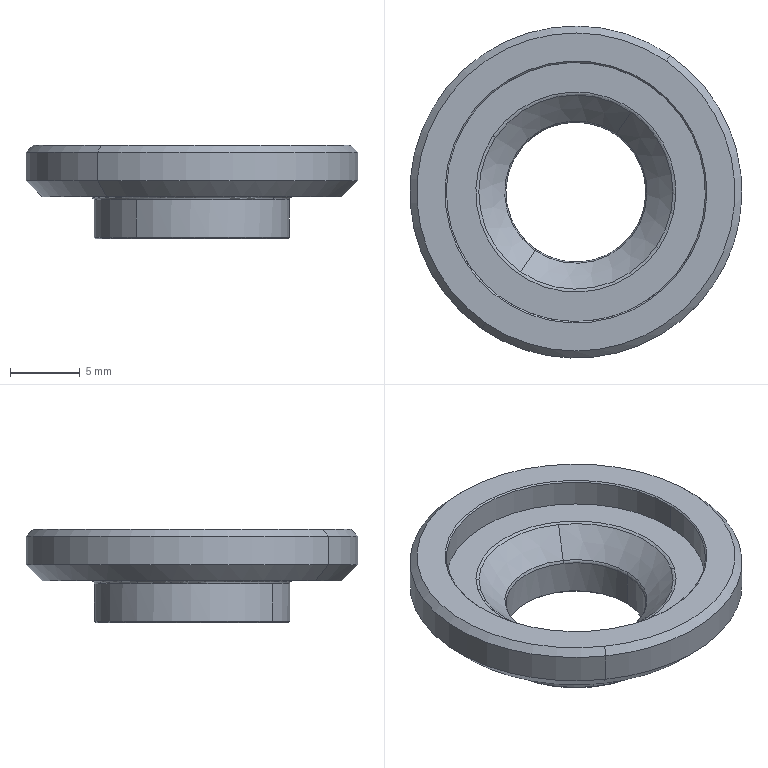Part | SolidWorks | features BaseBody 1 | 1 solid | 36 faces | box 23.8 x 23.8 x 6.7 mm | volume 1063 mm3 | cone 14 | cylinder 10 | torus 8 | plane 4 | commonest cylinder face diameters 14 x3 23.8 x3 10.04 x2 18.57 x2
STEP:
#1=CARTESIAN_POINT('',(85.216,-198.027,4.7));
#2=VERTEX_POINT('',#1);
#3=CARTESIAN_POINT('',(97.083,-206.078,4.7));
#4=VERTEX_POINT('',#3);
#5=CARTESIAN_POINT('',(91.15,-202.053,4.7));
#6=DIRECTION('',(0.,0.,1.));
#7=DIRECTION('',(-0.8275,0.5614,0.));
#8=AXIS2_PLACEMENT_3D('',#5,#6,#7);
#9=CIRCLE('',#8,7.17);
#10=EDGE_CURVE('',#2,#4,#9,.T.);
#11=ORIENTED_EDGE('',*,*,#10,.T.);
#12=CARTESIAN_POINT('',(96.907,-205.959,4.612));
#13=VERTEX_POINT('',#12);
#14=CARTESIAN_POINT('',(97.083,-206.078,4.4));
#15=DIRECTION('',(0.5614,0.8275,0.));
#16=DIRECTION('',(-0.5851,0.397,0.7071));
#17=AXIS2_PLACEMENT_3D('',#14,#15,#16);
#18=CIRCLE('',#17,0.3);
#19=EDGE_CURVE('',#13,#4,#18,.T.);
#20=ORIENTED_EDGE('',*,*,#19,.F.);
#21=CARTESIAN_POINT('',(87.195,-207.777,4.612));
#22=VERTEX_POINT('',#21);
#23=CARTESIAN_POINT('',(91.15,-202.053,4.612));
#24=DIRECTION('',(0.,0.,1.));
#25=DIRECTION('',(-0.5684,-0.8228,0.));
#26=AXIS2_PLACEMENT_3D('',#23,#24,#25);
#27=CIRCLE('',#26,6.958);
#28=EDGE_CURVE('',#22,#13,#27,.T.);
#29=ORIENTED_EDGE('',*,*,#28,.F.);
#30=CARTESIAN_POINT('',(85.392,-198.147,4.612));
#31=VERTEX_POINT('',#30);
#32=CARTESIAN_POINT('',(91.15,-202.053,4.612));
#33=DIRECTION('',(0.,0.,1.));
#34=DIRECTION('',(-0.8275,0.5614,0.));
#35=AXIS2_PLACEMENT_3D('',#32,#33,#34);
#36=CIRCLE('',#35,6.958);
#37=EDGE_CURVE('',#31,#22,#36,.T.);
#38=ORIENTED_EDGE('',*,*,#37,.F.);
#39=CARTESIAN_POINT('',(85.216,-198.027,4.4));
#40=DIRECTION('',(0.5614,0.8275,0.));
#41=DIRECTION('',(0.,0.,1.));
#42=AXIS2_PLACEMENT_3D('',#39,#40,#41);
#43=CIRCLE('',#42,0.3);
#44=EDGE_CURVE('',#2,#31,#43,.T.);
#45=ORIENTED_EDGE('',*,*,#44,.F.);
#46=EDGE_LOOP('',(#11,#20,#29,#38,#45));
#47=FACE_OUTER_BOUND('',#46,.T.);
#48=CARTESIAN_POINT('',(91.15,-202.053,4.4));
#49=DIRECTION('',(0.,0.,-1.));
#50=DIRECTION('',(0.8275,-0.5614,0.));
#51=AXIS2_PLACEMENT_3D('',#48,#49,#50);
#52=TOROIDAL_SURFACE('',#51,7.17,0.3);
#53=ADVANCED_FACE('',(#47),#52,.T.);
#54=ORIENTED_EDGE('',*,*,#44,.T.);
#55=CARTESIAN_POINT('',(95.104,-196.328,4.612));
#56=VERTEX_POINT('',#55);
#57=CARTESIAN_POINT('',(91.15,-202.053,4.612));
#58=DIRECTION('',(0.,0.,1.));
#59=DIRECTION('',(0.5684,0.8228,0.));
#60=AXIS2_PLACEMENT_3D('',#57,#58,#59);
#61=CIRCLE('',#60,6.958);
#62=EDGE_CURVE('',#56,#31,#61,.T.);
#63=ORIENTED_EDGE('',*,*,#62,.F.);
#64=CARTESIAN_POINT('',(91.15,-202.053,4.612));
#65=DIRECTION('',(0.,0.,1.));
#66=DIRECTION('',(0.8275,-0.5614,0.));
#67=AXIS2_PLACEMENT_3D('',#64,#65,#66);
#68=CIRCLE('',#67,6.958);
#69=EDGE_CURVE('',#13,#56,#68,.T.);
#70=ORIENTED_EDGE('',*,*,#69,.F.);
#71=ORIENTED_EDGE('',*,*,#19,.T.);
#72=CARTESIAN_POINT('',(91.15,-202.053,4.7));
#73=DIRECTION('',(0.,0.,1.));
#74=DIRECTION('',(0.8275,-0.5614,0.));
#75=AXIS2_PLACEMENT_3D('',#72,#73,#74);
#76=CIRCLE('',#75,7.17);
#77=EDGE_CURVE('',#4,#2,#76,.T.);
#78=ORIENTED_EDGE('',*,*,#77,.T.);
#79=EDGE_LOOP('',(#54,#63,#70,#71,#78));
#80=FACE_OUTER_BOUND('',#79,.T.);
#81=CARTESIAN_POINT('',(91.15,-202.053,4.4));
#82=DIRECTION('',(0.,0.,-1.));
#83=DIRECTION('',(-0.8275,0.5614,0.));
#84=AXIS2_PLACEMENT_3D('',#81,#82,#83);
#85=TOROIDAL_SURFACE('',#84,7.17,0.3);
#86=ADVANCED_FACE('',(#80),#85,.T.);
#87=ORIENTED_EDGE('',*,*,#77,.F.);
#88=ORIENTED_EDGE('',*,*,#10,.F.);
#89=EDGE_LOOP('',(#87,#88));
#90=FACE_BOUND('',#89,.T.);
#91=CARTESIAN_POINT('',(100.428,-202.4,4.7));
#92=VERTEX_POINT('',#91);
#93=CARTESIAN_POINT('',(81.871,-201.705,4.7));
#94=VERTEX_POINT('',#93);
#95=CARTESIAN_POINT('',(91.15,-202.053,4.7));
#96=DIRECTION('',(0.,0.,-1.));
#97=DIRECTION('',(0.9993,-0.03741,0.));
#98=AXIS2_PLACEMENT_3D('',#95,#96,#97);
#99=CIRCLE('',#98,9.285);
#100=EDGE_CURVE('',#92,#94,#99,.T.);
#101=ORIENTED_EDGE('',*,*,#100,.F.);
#102=CARTESIAN_POINT('',(91.15,-202.053,4.7));
#103=DIRECTION('',(0.,0.,-1.));
#104=DIRECTION('',(-0.9993,0.03741,0.));
#105=AXIS2_PLACEMENT_3D('',#102,#103,#104);
#106=CIRCLE('',#105,9.285);
#107=EDGE_CURVE('',#94,#92,#106,.T.);
#108=ORIENTED_EDGE('',*,*,#107,.F.);
#109=EDGE_LOOP('',(#101,#108));
#110=FACE_OUTER_BOUND('',#109,.T.);
#111=CARTESIAN_POINT('',(110.022,-194.263,4.7));
#112=DIRECTION('',(0.,0.,1.));
#113=DIRECTION('',(1.,0.,0.));
#114=AXIS2_PLACEMENT_3D('',#111,#112,#113);
#115=PLANE('',#114);
#116=ADVANCED_FACE('',(#90,#110),#115,.T.);
#117=CARTESIAN_POINT('',(81.871,-201.705,6.6));
#118=VERTEX_POINT('',#117);
#119=CARTESIAN_POINT('',(81.871,-201.705,6.6));
#120=DIRECTION('',(0.,0.,-1.));
#121=VECTOR('',#120,1000.);
#122=LINE('',#119,#121);
#123=EDGE_CURVE('',#118,#94,#122,.T.);
#124=ORIENTED_EDGE('',*,*,#123,.T.);
#125=ORIENTED_EDGE('',*,*,#107,.T.);
#126=CARTESIAN_POINT('',(100.428,-202.4,6.6));
#127=VERTEX_POINT('',#126);
#128=CARTESIAN_POINT('',(100.428,-202.4,6.6));
#129=DIRECTION('',(0.,0.,-1.));
#130=VECTOR('',#129,1000.);
#131=LINE('',#128,#130);
#132=EDGE_CURVE('',#127,#92,#131,.T.);
#133=ORIENTED_EDGE('',*,*,#132,.F.);
#134=CARTESIAN_POINT('',(91.15,-202.053,6.6));
#135=DIRECTION('',(0.,0.,1.));
#136=DIRECTION('',(0.9993,-0.03741,0.));
#137=AXIS2_PLACEMENT_3D('',#134,#135,#136);
#138=CIRCLE('',#137,9.285);
#139=EDGE_CURVE('',#127,#118,#138,.T.);
#140=ORIENTED_EDGE('',*,*,#139,.T.);
#141=EDGE_LOOP('',(#124,#125,#133,#140));
#142=FACE_OUTER_BOUND('',#141,.T.);
#143=CARTESIAN_POINT('',(91.15,-202.053,6.7));
#144=DIRECTION('',(0.,0.,1.));
#145=DIRECTION('',(0.9993,-0.03741,0.));
#146=AXIS2_PLACEMENT_3D('',#143,#144,#145);
#147=CYLINDRICAL_SURFACE('',#146,9.285);
#148=ADVANCED_FACE('',(#142),#147,.F.);
#149=CARTESIAN_POINT('',(81.771,-201.702,6.7));
#150=VERTEX_POINT('',#149);
#151=CARTESIAN_POINT('',(81.771,-201.702,6.7));
#152=DIRECTION('',(0.7066,-0.02645,-0.7071));
#153=VECTOR('',#152,1000.);
#154=LINE('',#151,#153);
#155=EDGE_CURVE('',#150,#118,#154,.T.);
#156=ORIENTED_EDGE('',*,*,#155,.T.);
#157=ORIENTED_EDGE('',*,*,#139,.F.);
#158=CARTESIAN_POINT('',(100.528,-202.404,6.7));
#159=VERTEX_POINT('',#158);
#160=CARTESIAN_POINT('',(100.528,-202.404,6.7));
#161=DIRECTION('',(-0.7066,0.02645,-0.7071));
#162=VECTOR('',#161,1000.);
#163=LINE('',#160,#162);
#164=EDGE_CURVE('',#159,#127,#163,.T.);
#165=ORIENTED_EDGE('',*,*,#164,.F.);
#166=CARTESIAN_POINT('',(91.15,-202.053,6.7));
#167=DIRECTION('',(0.,0.,1.));
#168=DIRECTION('',(0.9993,-0.03741,0.));
#169=AXIS2_PLACEMENT_3D('',#166,#167,#168);
#170=CIRCLE('',#169,9.385);
#171=EDGE_CURVE('',#159,#150,#170,.T.);
#172=ORIENTED_EDGE('',*,*,#171,.T.);
#173=EDGE_LOOP('',(#156,#157,#165,#172));
#174=FACE_OUTER_BOUND('',#173,.T.);
#175=CARTESIAN_POINT('',(91.15,-202.053,6.65));
#176=DIRECTION('',(0.,0.,1.));
#177=DIRECTION('',(-0.03741,-0.9993,0.));
#178=AXIS2_PLACEMENT_3D('',#175,#176,#177);
#179=CONICAL_SURFACE('',#178,9.335,0.7854);
#180=ADVANCED_FACE('',(#174),#179,.F.);
#181=CARTESIAN_POINT('',(90.799,-211.431,6.7));
#182=VERTEX_POINT('',#181);
#183=CARTESIAN_POINT('',(91.15,-202.053,6.7));
#184=DIRECTION('',(0.,0.,1.));
#185=DIRECTION('',(-0.03741,-0.9993,0.));
#186=AXIS2_PLACEMENT_3D('',#183,#184,#185);
#187=CIRCLE('',#186,9.385);
#188=EDGE_CURVE('',#150,#182,#187,.T.);
#189=ORIENTED_EDGE('',*,*,#188,.F.);
#190=ORIENTED_EDGE('',*,*,#171,.F.);
#191=CARTESIAN_POINT('',(91.15,-202.053,6.7));
#192=DIRECTION('',(0.,0.,1.));
#193=DIRECTION('',(-0.03741,-0.9993,0.));
#194=AXIS2_PLACEMENT_3D('',#191,#192,#193);
#195=CIRCLE('',#194,9.385);
#196=EDGE_CURVE('',#182,#159,#195,.T.);
#197=ORIENTED_EDGE('',*,*,#196,.F.);
#198=EDGE_LOOP('',(#189,#190,#197));
#199=FACE_BOUND('',#198,.T.);
#200=CARTESIAN_POINT('',(84.67,-211.432,6.7));
#201=VERTEX_POINT('',#200);
#202=CARTESIAN_POINT('',(97.629,-192.673,6.7));
#203=VERTEX_POINT('',#202);
#204=CARTESIAN_POINT('',(91.15,-202.053,6.7));
#205=DIRECTION('',(0.,0.,-1.));
#206=DIRECTION('',(-0.8228,0.5684,0.));
#207=AXIS2_PLACEMENT_3D('',#204,#205,#206);
#208=CIRCLE('',#207,11.4);
#209=EDGE_CURVE('',#201,#203,#208,.T.);
#210=ORIENTED_EDGE('',*,*,#209,.F.);
#211=CARTESIAN_POINT('',(91.15,-202.053,6.7));
#212=DIRECTION('',(0.,0.,-1.));
#213=DIRECTION('',(0.8228,-0.5684,0.));
#214=AXIS2_PLACEMENT_3D('',#211,#212,#213);
#215=CIRCLE('',#214,11.4);
#216=EDGE_CURVE('',#203,#201,#215,.T.);
#217=ORIENTED_EDGE('',*,*,#216,.F.);
#218=EDGE_LOOP('',(#210,#217));
#219=FACE_OUTER_BOUND('',#218,.T.);
#220=CARTESIAN_POINT('',(94.63,-221.084,6.7));
#221=DIRECTION('',(0.,0.,1.));
#222=DIRECTION('',(1.,0.,0.));
#223=AXIS2_PLACEMENT_3D('',#220,#221,#222);
#224=PLANE('',#223);
#225=ADVANCED_FACE('',(#199,#219),#224,.T.);
#226=CARTESIAN_POINT('',(97.913,-192.262,6.2));
#227=VERTEX_POINT('',#226);
#228=CARTESIAN_POINT('',(97.629,-192.673,6.7));
#229=DIRECTION('',(0.4019,0.5818,-0.7071));
#230=VECTOR('',#229,1000.);
#231=LINE('',#228,#230);
#232=EDGE_CURVE('',#203,#227,#231,.T.);
#233=ORIENTED_EDGE('',*,*,#232,.F.);
#234=ORIENTED_EDGE('',*,*,#216,.T.);
#235=CARTESIAN_POINT('',(84.386,-211.844,6.2));
#236=VERTEX_POINT('',#235);
#237=CARTESIAN_POINT('',(84.386,-211.844,6.2));
#238=DIRECTION('',(0.4019,0.5818,0.7071));
#239=VECTOR('',#238,1000.);
#240=LINE('',#237,#239);
#241=EDGE_CURVE('',#236,#201,#240,.T.);
#242=ORIENTED_EDGE('',*,*,#241,.F.);
#243=CARTESIAN_POINT('',(103.041,-202.498,6.2));
#244=VERTEX_POINT('',#243);
#245=CARTESIAN_POINT('',(91.15,-202.053,6.2));
#246=DIRECTION('',(0.,0.,-1.));
#247=DIRECTION('',(0.8228,-0.5684,0.));
#248=AXIS2_PLACEMENT_3D('',#245,#246,#247);
#249=CIRCLE('',#248,11.9);
#250=EDGE_CURVE('',#244,#236,#249,.T.);
#251=ORIENTED_EDGE('',*,*,#250,.F.);
#252=CARTESIAN_POINT('',(91.15,-202.053,6.2));
#253=DIRECTION('',(0.,0.,-1.));
#254=DIRECTION('',(0.8228,-0.5684,0.));
#255=AXIS2_PLACEMENT_3D('',#252,#253,#254);
#256=CIRCLE('',#255,11.9);
#257=EDGE_CURVE('',#227,#244,#256,.T.);
#258=ORIENTED_EDGE('',*,*,#257,.F.);
#259=EDGE_LOOP('',(#233,#234,#242,#251,#258));
#260=FACE_OUTER_BOUND('',#259,.T.);
#261=CARTESIAN_POINT('',(91.15,-202.053,6.45));
#262=DIRECTION('',(0.,0.,-1.));
#263=DIRECTION('',(-0.8228,0.5684,0.));
#264=AXIS2_PLACEMENT_3D('',#261,#262,#263);
#265=CONICAL_SURFACE('',#264,11.65,0.7854);
#266=ADVANCED_FACE('',(#260),#265,.T.);
#267=ORIENTED_EDGE('',*,*,#232,.T.);
#268=CARTESIAN_POINT('',(91.15,-202.053,6.2));
#269=DIRECTION('',(0.,0.,-1.));
#270=DIRECTION('',(-0.8228,0.5684,0.));
#271=AXIS2_PLACEMENT_3D('',#268,#269,#270);
#272=CIRCLE('',#271,11.9);
#273=EDGE_CURVE('',#236,#227,#272,.T.);
#274=ORIENTED_EDGE('',*,*,#273,.F.);
#275=ORIENTED_EDGE('',*,*,#241,.T.);
#276=ORIENTED_EDGE('',*,*,#209,.T.);
#277=EDGE_LOOP('',(#267,#274,#275,#276));
#278=FACE_OUTER_BOUND('',#277,.T.);
#279=CARTESIAN_POINT('',(91.15,-202.053,6.45));
#280=DIRECTION('',(0.,0.,-1.));
#281=DIRECTION('',(0.8228,-0.5684,0.));
#282=AXIS2_PLACEMENT_3D('',#279,#280,#281);
#283=CONICAL_SURFACE('',#282,11.65,0.7854);
#284=ADVANCED_FACE('',(#278),#283,.T.);
#285=CARTESIAN_POINT('',(97.913,-192.262,4.15));
#286=VERTEX_POINT('',#285);
#287=CARTESIAN_POINT('',(84.386,-211.844,4.15));
#288=VERTEX_POINT('',#287);
#289=CARTESIAN_POINT('',(91.15,-202.053,4.15));
#290=DIRECTION('',(0.,0.,1.));
#291=DIRECTION('',(-0.8228,0.5684,0.));
#292=AXIS2_PLACEMENT_3D('',#289,#290,#291);
#293=CIRCLE('',#292,11.9);
#294=EDGE_CURVE('',#286,#288,#293,.T.);
#295=ORIENTED_EDGE('',*,*,#294,.T.);
#296=CARTESIAN_POINT('',(84.386,-211.844,4.15));
#297=DIRECTION('',(0.,0.,1.));
#298=VECTOR('',#297,1000.);
#299=LINE('',#296,#298);
#300=EDGE_CURVE('',#288,#236,#299,.T.);
#301=ORIENTED_EDGE('',*,*,#300,.T.);
#302=ORIENTED_EDGE('',*,*,#273,.T.);
#303=CARTESIAN_POINT('',(97.913,-192.262,6.2));
#304=DIRECTION('',(0.,0.,-1.));
#305=VECTOR('',#304,1000.);
#306=LINE('',#303,#305);
#307=EDGE_CURVE('',#227,#286,#306,.T.);
#308=ORIENTED_EDGE('',*,*,#307,.T.);
#309=EDGE_LOOP('',(#295,#301,#302,#308));
#310=FACE_OUTER_BOUND('',#309,.T.);
#311=CARTESIAN_POINT('',(91.15,-202.053,5.175));
#312=DIRECTION('',(0.,0.,1.));
#313=DIRECTION('',(0.9993,-0.03741,0.));
#314=AXIS2_PLACEMENT_3D('',#311,#312,#313);
#315=CYLINDRICAL_SURFACE('',#314,11.9);
#316=ADVANCED_FACE('',(#310),#315,.T.);
#317=CARTESIAN_POINT('',(97.26,-193.208,3.));
#318=VERTEX_POINT('',#317);
#319=CARTESIAN_POINT('',(85.04,-210.898,3.));
#320=VERTEX_POINT('',#319);
#321=CARTESIAN_POINT('',(91.15,-202.053,3.));
#322=DIRECTION('',(0.,0.,1.));
#323=DIRECTION('',(-0.8228,0.5684,0.));
#324=AXIS2_PLACEMENT_3D('',#321,#322,#323);
#325=CIRCLE('',#324,10.75);
#326=EDGE_CURVE('',#318,#320,#325,.T.);
#327=ORIENTED_EDGE('',*,*,#326,.T.);
#328=CARTESIAN_POINT('',(85.04,-210.898,3.));
#329=DIRECTION('',(-0.4019,-0.5818,0.7071));
#330=VECTOR('',#329,1000.);
#331=LINE('',#328,#330);
#332=EDGE_CURVE('',#320,#288,#331,.T.);
#333=ORIENTED_EDGE('',*,*,#332,.T.);
#334=ORIENTED_EDGE('',*,*,#294,.F.);
#335=CARTESIAN_POINT('',(97.913,-192.262,4.15));
#336=DIRECTION('',(-0.4019,-0.5818,-0.7071));
#337=VECTOR('',#336,1000.);
#338=LINE('',#335,#337);
#339=EDGE_CURVE('',#286,#318,#338,.T.);
#340=ORIENTED_EDGE('',*,*,#339,.T.);
#341=EDGE_LOOP('',(#327,#333,#334,#340));
#342=FACE_OUTER_BOUND('',#341,.T.);
#343=CARTESIAN_POINT('',(91.15,-202.053,3.575));
#344=DIRECTION('',(0.,0.,1.));
#345=DIRECTION('',(0.8228,-0.5684,0.));
#346=AXIS2_PLACEMENT_3D('',#343,#344,#345);
#347=CONICAL_SURFACE('',#346,11.325,0.7854);
#348=ADVANCED_FACE('',(#342),#347,.T.);
#349=CARTESIAN_POINT('',(97.074,-206.145,3.));
#350=VERTEX_POINT('',#349);
#351=CARTESIAN_POINT('',(85.182,-198.024,3.));
#352=VERTEX_POINT('',#351);
#353=CARTESIAN_POINT('',(91.15,-202.053,3.));
#354=DIRECTION('',(0.,0.,-1.));
#355=DIRECTION('',(0.8228,-0.5683,0.));
#356=AXIS2_PLACEMENT_3D('',#353,#354,#355);
#357=CIRCLE('',#356,7.2);
#358=EDGE_CURVE('',#350,#352,#357,.T.);
#359=ORIENTED_EDGE('',*,*,#358,.F.);
#360=CARTESIAN_POINT('',(97.117,-206.082,3.));
#361=VERTEX_POINT('',#360);
#362=CARTESIAN_POINT('',(91.15,-202.053,3.));
#363=DIRECTION('',(0.,0.,-1.));
#364=DIRECTION('',(0.8288,-0.5596,0.));
#365=AXIS2_PLACEMENT_3D('',#362,#363,#364);
#366=CIRCLE('',#365,7.2);
#367=EDGE_CURVE('',#361,#350,#366,.T.);
#368=ORIENTED_EDGE('',*,*,#367,.F.);
#369=CARTESIAN_POINT('',(85.225,-197.961,3.));
#370=VERTEX_POINT('',#369);
#371=CARTESIAN_POINT('',(91.15,-202.053,3.));
#372=DIRECTION('',(0.,0.,-1.));
#373=DIRECTION('',(-0.8228,0.5683,0.));
#374=AXIS2_PLACEMENT_3D('',#371,#372,#373);
#375=CIRCLE('',#374,7.2);
#376=EDGE_CURVE('',#370,#361,#375,.T.);
#377=ORIENTED_EDGE('',*,*,#376,.F.);
#378=CARTESIAN_POINT('',(91.15,-202.053,3.));
#379=DIRECTION('',(0.,0.,-1.));
#380=DIRECTION('',(-0.8288,0.5596,0.));
#381=AXIS2_PLACEMENT_3D('',#378,#379,#380);
#382=CIRCLE('',#381,7.2);
#383=EDGE_CURVE('',#352,#370,#382,.T.);
#384=ORIENTED_EDGE('',*,*,#383,.F.);
#385=EDGE_LOOP('',(#359,#368,#377,#384));
#386=FACE_BOUND('',#385,.T.);
#387=ORIENTED_EDGE('',*,*,#326,.F.);
#388=CARTESIAN_POINT('',(91.15,-202.053,3.));
#389=DIRECTION('',(0.,0.,1.));
#390=DIRECTION('',(0.8228,-0.5684,0.));
#391=AXIS2_PLACEMENT_3D('',#388,#389,#390);
#392=CIRCLE('',#391,10.75);
#393=EDGE_CURVE('',#320,#318,#392,.T.);
#394=ORIENTED_EDGE('',*,*,#393,.F.);
#395=EDGE_LOOP('',(#387,#394));
#396=FACE_OUTER_BOUND('',#395,.T.);
#397=CARTESIAN_POINT('',(91.994,-223.527,3.));
#398=DIRECTION('',(0.,0.,-1.));
#399=DIRECTION('',(0.,-1.,0.));
#400=AXIS2_PLACEMENT_3D('',#397,#398,#399);
#401=PLANE('',#400);
#402=ADVANCED_FACE('',(#386,#396),#401,.T.);
#403=ORIENTED_EDGE('',*,*,#332,.F.);
#404=ORIENTED_EDGE('',*,*,#393,.T.);
#405=ORIENTED_EDGE('',*,*,#339,.F.);
#406=CARTESIAN_POINT('',(103.041,-202.498,4.15));
#407=VERTEX_POINT('',#406);
#408=CARTESIAN_POINT('',(91.15,-202.053,4.15));
#409=DIRECTION('',(0.,0.,1.));
#410=DIRECTION('',(0.9993,-0.03741,0.));
#411=AXIS2_PLACEMENT_3D('',#408,#409,#410);
#412=CIRCLE('',#411,11.9);
#413=EDGE_CURVE('',#407,#286,#412,.T.);
#414=ORIENTED_EDGE('',*,*,#413,.F.);
#415=CARTESIAN_POINT('',(91.15,-202.053,4.15));
#416=DIRECTION('',(0.,0.,1.));
#417=DIRECTION('',(0.9993,-0.03741,0.));
#418=AXIS2_PLACEMENT_3D('',#415,#416,#417);
#419=CIRCLE('',#418,11.9);
#420=EDGE_CURVE('',#288,#407,#419,.T.);
#421=ORIENTED_EDGE('',*,*,#420,.F.);
#422=EDGE_LOOP('',(#403,#404,#405,#414,#421));
#423=FACE_OUTER_BOUND('',#422,.T.);
#424=CARTESIAN_POINT('',(91.15,-202.053,3.575));
#425=DIRECTION('',(0.,0.,1.));
#426=DIRECTION('',(-0.8228,0.5684,0.));
#427=AXIS2_PLACEMENT_3D('',#424,#425,#426);
#428=CONICAL_SURFACE('',#427,11.325,0.7854);
#429=ADVANCED_FACE('',(#423),#428,.T.);
#430=CARTESIAN_POINT('',(103.041,-202.498,5.175));
#431=DIRECTION('',(0.,0.,1.));
#432=VECTOR('',#431,1000.);
#433=LINE('',#430,#432);
#434=EDGE_CURVE('',#407,#244,#433,.T.);
#435=ORIENTED_EDGE('',*,*,#434,.F.);
#436=ORIENTED_EDGE('',*,*,#413,.T.);
#437=ORIENTED_EDGE('',*,*,#307,.F.);
#438=ORIENTED_EDGE('',*,*,#257,.T.);
#439=EDGE_LOOP('',(#435,#436,#437,#438));
#440=FACE_OUTER_BOUND('',#439,.T.);
#441=CARTESIAN_POINT('',(91.15,-202.053,5.175));
#442=DIRECTION('',(0.,0.,1.));
#443=DIRECTION('',(0.9993,-0.03741,0.));
#444=AXIS2_PLACEMENT_3D('',#441,#442,#443);
#445=CYLINDRICAL_SURFACE('',#444,11.9);
#446=ADVANCED_FACE('',(#440),#445,.T.);
#447=ORIENTED_EDGE('',*,*,#383,.T.);
#448=ORIENTED_EDGE('',*,*,#376,.T.);
#449=CARTESIAN_POINT('',(96.951,-205.969,2.8));
#450=VERTEX_POINT('',#449);
#451=CARTESIAN_POINT('',(97.117,-206.081,2.8));
#452=DIRECTION('',(0.5595,0.8288,0.));
#453=DIRECTION('',(-0.8288,0.5595,0.));
#454=AXIS2_PLACEMENT_3D('',#451,#452,#453);
#455=CIRCLE('',#454,0.2);
#456=EDGE_CURVE('',#450,#361,#455,.T.);
#457=ORIENTED_EDGE('',*,*,#456,.F.);
#458=CARTESIAN_POINT('',(98.145,-202.315,2.8));
#459=VERTEX_POINT('',#458);
#460=CARTESIAN_POINT('',(91.15,-202.053,2.8));
#461=DIRECTION('',(0.,0.,-1.));
#462=DIRECTION('',(0.9993,-0.03741,0.));
#463=AXIS2_PLACEMENT_3D('',#460,#461,#462);
#464=CIRCLE('',#463,7.);
#465=EDGE_CURVE('',#459,#450,#464,.T.);
#466=ORIENTED_EDGE('',*,*,#465,.F.);
#467=CARTESIAN_POINT('',(95.128,-196.293,2.8));
#468=VERTEX_POINT('',#467);
#469=CARTESIAN_POINT('',(91.15,-202.053,2.8));
#470=DIRECTION('',(0.,0.,-1.));
#471=DIRECTION('',(0.9993,-0.03741,0.));
#472=AXIS2_PLACEMENT_3D('',#469,#470,#471);
#473=CIRCLE('',#472,7.);
#474=EDGE_CURVE('',#468,#459,#473,.T.);
#475=ORIENTED_EDGE('',*,*,#474,.F.);
#476=CARTESIAN_POINT('',(85.348,-198.136,2.8));
#477=VERTEX_POINT('',#476);
#478=CARTESIAN_POINT('',(91.15,-202.053,2.8));
#479=DIRECTION('',(0.,0.,-1.));
#480=DIRECTION('',(-0.8288,0.5595,0.));
#481=AXIS2_PLACEMENT_3D('',#478,#479,#480);
#482=CIRCLE('',#481,7.);
#483=EDGE_CURVE('',#477,#468,#482,.T.);
#484=ORIENTED_EDGE('',*,*,#483,.F.);
#485=CARTESIAN_POINT('',(85.182,-198.024,2.8));
#486=DIRECTION('',(0.5595,0.8288,0.));
#487=DIRECTION('',(0.000000717,-0.000000484,1.));
#488=AXIS2_PLACEMENT_3D('',#485,#486,#487);
#489=CIRCLE('',#488,0.2);
#490=EDGE_CURVE('',#352,#477,#489,.T.);
#491=ORIENTED_EDGE('',*,*,#490,.F.);
#492=EDGE_LOOP('',(#447,#448,#457,#466,#475,#484,#491));
#493=FACE_OUTER_BOUND('',#492,.T.);
#494=CARTESIAN_POINT('',(91.15,-202.053,2.8));
#495=DIRECTION('',(0.,0.,1.));
#496=DIRECTION('',(0.8288,-0.5595,0.));
#497=AXIS2_PLACEMENT_3D('',#494,#495,#496);
#498=TOROIDAL_SURFACE('',#497,7.2,0.2);
#499=ADVANCED_FACE('',(#493),#498,.F.);
#500=CARTESIAN_POINT('',(87.171,-207.812,2.8));
#501=VERTEX_POINT('',#500);
#502=CARTESIAN_POINT('',(91.15,-202.053,2.8));
#503=DIRECTION('',(0.,0.,-1.));
#504=DIRECTION('',(-0.5684,-0.8228,0.));
#505=AXIS2_PLACEMENT_3D('',#502,#503,#504);
#506=CIRCLE('',#505,7.);
#507=EDGE_CURVE('',#501,#477,#506,.T.);
#508=ORIENTED_EDGE('',*,*,#507,.F.);
#509=CARTESIAN_POINT('',(91.15,-202.053,2.8));
#510=DIRECTION('',(0.,0.,-1.));
#511=DIRECTION('',(0.8288,-0.5595,0.));
#512=AXIS2_PLACEMENT_3D('',#509,#510,#511);
#513=CIRCLE('',#512,7.);
#514=EDGE_CURVE('',#450,#501,#513,.T.);
#515=ORIENTED_EDGE('',*,*,#514,.F.);
#516=ORIENTED_EDGE('',*,*,#456,.T.);
#517=ORIENTED_EDGE('',*,*,#367,.T.);
#518=ORIENTED_EDGE('',*,*,#358,.T.);
#519=ORIENTED_EDGE('',*,*,#490,.T.);
#520=EDGE_LOOP('',(#508,#515,#516,#517,#518,#519));
#521=FACE_OUTER_BOUND('',#520,.T.);
#522=CARTESIAN_POINT('',(91.15,-202.053,2.8));
#523=DIRECTION('',(0.,0.,1.));
#524=DIRECTION('',(-0.8288,0.5595,0.));
#525=AXIS2_PLACEMENT_3D('',#522,#523,#524);
#526=TOROIDAL_SURFACE('',#525,7.2,0.2);
#527=ADVANCED_FACE('',(#521),#526,.F.);
#528=CARTESIAN_POINT('',(95.128,-196.293,0.1));
#529=VERTEX_POINT('',#528);
#530=CARTESIAN_POINT('',(87.171,-207.812,0.1));
#531=VERTEX_POINT('',#530);
#532=CARTESIAN_POINT('',(91.15,-202.053,0.1));
#533=DIRECTION('',(0.,0.,1.));
#534=DIRECTION('',(-0.8228,0.5684,0.));
#535=AXIS2_PLACEMENT_3D('',#532,#533,#534);
#536=CIRCLE('',#535,7.);
#537=EDGE_CURVE('',#529,#531,#536,.T.);
#538=ORIENTED_EDGE('',*,*,#537,.T.);
#539=CARTESIAN_POINT('',(87.171,-207.812,0.1));
#540=DIRECTION('',(-0.000006304,0.000004355,1.));
#541=VECTOR('',#540,1000.);
#542=LINE('',#539,#541);
#543=EDGE_CURVE('',#531,#501,#542,.T.);
#544=ORIENTED_EDGE('',*,*,#543,.T.);
#545=ORIENTED_EDGE('',*,*,#507,.T.);
#546=ORIENTED_EDGE('',*,*,#483,.T.);
#547=CARTESIAN_POINT('',(95.128,-196.293,2.8));
#548=DIRECTION('',(-0.000004649,0.000003212,-1.));
#549=VECTOR('',#548,1000.);
#550=LINE('',#547,#549);
#551=EDGE_CURVE('',#468,#529,#550,.T.);
#552=ORIENTED_EDGE('',*,*,#551,.T.);
#553=EDGE_LOOP('',(#538,#544,#545,#546,#552));
#554=FACE_OUTER_BOUND('',#553,.T.);
#555=CARTESIAN_POINT('',(91.15,-202.053,1.45));
#556=DIRECTION('',(0.,0.,1.));
#557=DIRECTION('',(0.9993,-0.03741,0.));
#558=AXIS2_PLACEMENT_3D('',#555,#556,#557);
#559=CYLINDRICAL_SURFACE('',#558,7.);
#560=ADVANCED_FACE('',(#554),#559,.T.);
#561=CARTESIAN_POINT('',(87.228,-207.73,0.));
#562=VERTEX_POINT('',#561);
#563=CARTESIAN_POINT('',(87.228,-207.73,0.));
#564=DIRECTION('',(-0.4021,-0.5817,0.7071));
#565=VECTOR('',#564,1000.);
#566=LINE('',#563,#565);
#567=EDGE_CURVE('',#562,#531,#566,.T.);
#568=ORIENTED_EDGE('',*,*,#567,.T.);
#569=ORIENTED_EDGE('',*,*,#537,.F.);
#570=CARTESIAN_POINT('',(95.071,-196.376,0.));
#571=VERTEX_POINT('',#570);
#572=CARTESIAN_POINT('',(95.128,-196.293,0.1));
#573=DIRECTION('',(-0.402,-0.5817,-0.7071));
#574=VECTOR('',#573,1000.);
#575=LINE('',#572,#574);
#576=EDGE_CURVE('',#529,#571,#575,.T.);
#577=ORIENTED_EDGE('',*,*,#576,.T.);
#578=CARTESIAN_POINT('',(91.15,-202.053,0.));
#579=DIRECTION('',(0.,0.,1.));
#580=DIRECTION('',(0.5684,0.8228,0.));
#581=AXIS2_PLACEMENT_3D('',#578,#579,#580);
#582=CIRCLE('',#581,6.9);
#583=EDGE_CURVE('',#571,#562,#582,.T.);
#584=ORIENTED_EDGE('',*,*,#583,.T.);
#585=EDGE_LOOP('',(#568,#569,#577,#584));
#586=FACE_OUTER_BOUND('',#585,.T.);
#587=CARTESIAN_POINT('',(91.15,-202.053,0.05));
#588=DIRECTION('',(0.,0.,1.));
#589=DIRECTION('',(0.8228,-0.5684,0.));
#590=AXIS2_PLACEMENT_3D('',#587,#588,#589);
#591=CONICAL_SURFACE('',#590,6.95,0.7854);
#592=ADVANCED_FACE('',(#586),#591,.T.);
#593=CARTESIAN_POINT('',(96.266,-202.244,0.));
#594=VERTEX_POINT('',#593);
#595=CARTESIAN_POINT('',(90.958,-207.169,0.));
#596=VERTEX_POINT('',#595);
#597=CARTESIAN_POINT('',(91.15,-202.053,0.));
#598=DIRECTION('',(0.,0.,-1.));
#599=DIRECTION('',(-0.03741,-0.9993,0.));
#600=AXIS2_PLACEMENT_3D('',#597,#598,#599);
#601=CIRCLE('',#600,5.12);
#602=EDGE_CURVE('',#594,#596,#601,.T.);
#603=ORIENTED_EDGE('',*,*,#602,.F.);
#604=CARTESIAN_POINT('',(86.033,-201.861,0.));
#605=VERTEX_POINT('',#604);
#606=CARTESIAN_POINT('',(91.15,-202.053,0.));
#607=DIRECTION('',(0.,0.,-1.));
#608=DIRECTION('',(0.03741,0.9993,0.));
#609=AXIS2_PLACEMENT_3D('',#606,#607,#608);
#610=CIRCLE('',#609,5.12);
#611=EDGE_CURVE('',#605,#594,#610,.T.);
#612=ORIENTED_EDGE('',*,*,#611,.F.);
#613=CARTESIAN_POINT('',(91.15,-202.053,0.));
#614=DIRECTION('',(0.,0.,-1.));
#615=DIRECTION('',(-0.03741,-0.9993,0.));
#616=AXIS2_PLACEMENT_3D('',#613,#614,#615);
#617=CIRCLE('',#616,5.12);
#618=EDGE_CURVE('',#596,#605,#617,.T.);
#619=ORIENTED_EDGE('',*,*,#618,.F.);
#620=EDGE_LOOP('',(#603,#612,#619));
#621=FACE_BOUND('',#620,.T.);
#622=CARTESIAN_POINT('',(91.15,-202.053,0.));
#623=DIRECTION('',(0.,0.,1.));
#624=DIRECTION('',(0.8228,-0.5684,0.));
#625=AXIS2_PLACEMENT_3D('',#622,#623,#624);
#626=CIRCLE('',#625,6.9);
#627=EDGE_CURVE('',#562,#571,#626,.T.);
#628=ORIENTED_EDGE('',*,*,#627,.F.);
#629=ORIENTED_EDGE('',*,*,#583,.F.);
#630=EDGE_LOOP('',(#628,#629));
#631=FACE_OUTER_BOUND('',#630,.T.);
#632=CARTESIAN_POINT('',(93.256,-213.572,0.));
#633=DIRECTION('',(0.,0.,-1.));
#634=DIRECTION('',(0.,-1.,0.));
#635=AXIS2_PLACEMENT_3D('',#632,#633,#634);
#636=PLANE('',#635);
#637=ADVANCED_FACE('',(#621,#631),#636,.T.);
#638=ORIENTED_EDGE('',*,*,#567,.F.);
#639=ORIENTED_EDGE('',*,*,#627,.T.);
#640=ORIENTED_EDGE('',*,*,#576,.F.);
#641=CARTESIAN_POINT('',(98.145,-202.315,0.1));
#642=VERTEX_POINT('',#641);
#643=CARTESIAN_POINT('',(91.15,-202.053,0.1));
#644=DIRECTION('',(0.,0.,1.));
#645=DIRECTION('',(0.9993,-0.03741,0.));
#646=AXIS2_PLACEMENT_3D('',#643,#644,#645);
#647=CIRCLE('',#646,7.);
#648=EDGE_CURVE('',#642,#529,#647,.T.);
#649=ORIENTED_EDGE('',*,*,#648,.F.);
#650=CARTESIAN_POINT('',(91.15,-202.053,0.1));
#651=DIRECTION('',(0.,0.,1.));
#652=DIRECTION('',(0.9993,-0.03741,0.));
#653=AXIS2_PLACEMENT_3D('',#650,#651,#652);
#654=CIRCLE('',#653,7.);
#655=EDGE_CURVE('',#531,#642,#654,.T.);
#656=ORIENTED_EDGE('',*,*,#655,.F.);
#657=EDGE_LOOP('',(#638,#639,#640,#649,#656));
#658=FACE_OUTER_BOUND('',#657,.T.);
#659=CARTESIAN_POINT('',(91.15,-202.053,0.05));
#660=DIRECTION('',(0.,0.,1.));
#661=DIRECTION('',(-0.8228,0.5684,0.));
#662=AXIS2_PLACEMENT_3D('',#659,#660,#661);
#663=CONICAL_SURFACE('',#662,6.95,0.7854);
#664=ADVANCED_FACE('',(#658),#663,.T.);
#665=CARTESIAN_POINT('',(98.145,-202.315,1.45));
#666=DIRECTION('',(0.,0.,1.));
#667=VECTOR('',#666,1000.);
#668=LINE('',#665,#667);
#669=EDGE_CURVE('',#642,#459,#668,.T.);
#670=ORIENTED_EDGE('',*,*,#669,.F.);
#671=ORIENTED_EDGE('',*,*,#648,.T.);
#672=ORIENTED_EDGE('',*,*,#551,.F.);
#673=ORIENTED_EDGE('',*,*,#474,.T.);
#674=EDGE_LOOP('',(#670,#671,#672,#673));
#675=FACE_OUTER_BOUND('',#674,.T.);
#676=CARTESIAN_POINT('',(91.15,-202.053,1.45));
#677=DIRECTION('',(0.,0.,1.));
#678=DIRECTION('',(0.9993,-0.03741,0.));
#679=AXIS2_PLACEMENT_3D('',#676,#677,#678);
#680=CYLINDRICAL_SURFACE('',#679,7.);
#681=ADVANCED_FACE('',(#675),#680,.T.);
#682=CARTESIAN_POINT('',(96.166,-202.241,0.1));
#683=VERTEX_POINT('',#682);
#684=CARTESIAN_POINT('',(96.266,-202.244,0.));
#685=DIRECTION('',(-0.7066,0.02645,0.7071));
#686=VECTOR('',#685,1000.);
#687=LINE('',#684,#686);
#688=EDGE_CURVE('',#594,#683,#687,.T.);
#689=ORIENTED_EDGE('',*,*,#688,.T.);
#690=CARTESIAN_POINT('',(86.133,-201.865,0.1));
#691=VERTEX_POINT('',#690);
#692=CARTESIAN_POINT('',(91.15,-202.053,0.1));
#693=DIRECTION('',(0.,0.,-1.));
#694=DIRECTION('',(0.03741,0.9993,0.));
#695=AXIS2_PLACEMENT_3D('',#692,#693,#694);
#696=CIRCLE('',#695,5.02);
#697=EDGE_CURVE('',#691,#683,#696,.T.);
#698=ORIENTED_EDGE('',*,*,#697,.F.);
#699=CARTESIAN_POINT('',(86.033,-201.861,0.));
#700=DIRECTION('',(0.7066,-0.02645,0.7071));
#701=VECTOR('',#700,1000.);
#702=LINE('',#699,#701);
#703=EDGE_CURVE('',#605,#691,#702,.T.);
#704=ORIENTED_EDGE('',*,*,#703,.F.);
#705=ORIENTED_EDGE('',*,*,#611,.T.);
#706=EDGE_LOOP('',(#689,#698,#704,#705));
#707=FACE_OUTER_BOUND('',#706,.T.);
#708=CARTESIAN_POINT('',(91.15,-202.053,0.05));
#709=DIRECTION('',(0.,0.,-1.));
#710=DIRECTION('',(-0.03741,-0.9993,0.));
#711=AXIS2_PLACEMENT_3D('',#708,#709,#710);
#712=CONICAL_SURFACE('',#711,5.07,0.7854);
#713=ADVANCED_FACE('',(#707),#712,.F.);
#714=CARTESIAN_POINT('',(90.962,-207.069,0.1));
#715=VERTEX_POINT('',#714);
#716=CARTESIAN_POINT('',(90.96,-207.119,0.05));
#717=DIRECTION('',(-0.02645,-0.7066,-0.7071));
#718=VECTOR('',#717,1000.);
#719=LINE('',#716,#718);
#720=EDGE_CURVE('',#715,#596,#719,.T.);
#721=ORIENTED_EDGE('',*,*,#720,.F.);
#722=CARTESIAN_POINT('',(91.15,-202.053,0.1));
#723=DIRECTION('',(0.,0.,-1.));
#724=DIRECTION('',(-0.03741,-0.9993,0.));
#725=AXIS2_PLACEMENT_3D('',#722,#723,#724);
#726=CIRCLE('',#725,5.02);
#727=EDGE_CURVE('',#683,#715,#726,.T.);
#728=ORIENTED_EDGE('',*,*,#727,.F.);
#729=ORIENTED_EDGE('',*,*,#688,.F.);
#730=ORIENTED_EDGE('',*,*,#602,.T.);
#731=EDGE_LOOP('',(#721,#728,#729,#730));
#732=FACE_OUTER_BOUND('',#731,.T.);
#733=CARTESIAN_POINT('',(91.15,-202.053,0.05));
#734=DIRECTION('',(0.,0.,-1.));
#735=DIRECTION('',(-0.03741,-0.9993,0.));
#736=AXIS2_PLACEMENT_3D('',#733,#734,#735);
#737=CONICAL_SURFACE('',#736,5.07,0.7854);
#738=ADVANCED_FACE('',(#732),#737,.F.);
#739=CARTESIAN_POINT('',(86.133,-201.865,2.55));
#740=VERTEX_POINT('',#739);
#741=CARTESIAN_POINT('',(86.133,-201.865,0.1));
#742=DIRECTION('',(0.,0.,1.));
#743=VECTOR('',#742,1000.);
#744=LINE('',#741,#743);
#745=EDGE_CURVE('',#691,#740,#744,.T.);
#746=ORIENTED_EDGE('',*,*,#745,.T.);
#747=CARTESIAN_POINT('',(88.26,-206.158,2.55));
#748=VERTEX_POINT('',#747);
#749=CARTESIAN_POINT('',(91.15,-202.053,2.55));
#750=DIRECTION('',(0.,0.,1.));
#751=DIRECTION('',(-0.9993,0.03741,0.));
#752=AXIS2_PLACEMENT_3D('',#749,#750,#751);
#753=CIRCLE('',#752,5.02);
#754=EDGE_CURVE('',#740,#748,#753,.T.);
#755=ORIENTED_EDGE('',*,*,#754,.T.);
#756=CARTESIAN_POINT('',(88.296,-206.183,2.55));
#757=VERTEX_POINT('',#756);
#758=CARTESIAN_POINT('',(91.15,-202.053,2.55));
#759=DIRECTION('',(0.,0.,1.));
#760=DIRECTION('',(-0.9993,0.03741,0.));
#761=AXIS2_PLACEMENT_3D('',#758,#759,#760);
#762=CIRCLE('',#761,5.02);
#763=EDGE_CURVE('',#748,#757,#762,.T.);
#764=ORIENTED_EDGE('',*,*,#763,.T.);
#765=CARTESIAN_POINT('',(96.166,-202.241,2.55));
#766=VERTEX_POINT('',#765);
#767=CARTESIAN_POINT('',(91.15,-202.053,2.55));
#768=DIRECTION('',(0.,0.,1.));
#769=DIRECTION('',(-0.5684,-0.8228,0.));
#770=AXIS2_PLACEMENT_3D('',#767,#768,#769);
#771=CIRCLE('',#770,5.02);
#772=EDGE_CURVE('',#757,#766,#771,.T.);
#773=ORIENTED_EDGE('',*,*,#772,.T.);
#774=CARTESIAN_POINT('',(96.166,-202.241,0.1));
#775=DIRECTION('',(0.,0.,1.));
#776=VECTOR('',#775,1000.);
#777=LINE('',#774,#776);
#778=EDGE_CURVE('',#683,#766,#777,.T.);
#779=ORIENTED_EDGE('',*,*,#778,.F.);
#780=ORIENTED_EDGE('',*,*,#727,.T.);
#781=CARTESIAN_POINT('',(91.15,-202.053,0.1));
#782=DIRECTION('',(0.,0.,-1.));
#783=DIRECTION('',(-0.03741,-0.9993,0.));
#784=AXIS2_PLACEMENT_3D('',#781,#782,#783);
#785=CIRCLE('',#784,5.02);
#786=EDGE_CURVE('',#715,#691,#785,.T.);
#787=ORIENTED_EDGE('',*,*,#786,.T.);
#788=EDGE_LOOP('',(#746,#755,#764,#773,#779,#780,#787));
#789=FACE_OUTER_BOUND('',#788,.T.);
#790=CARTESIAN_POINT('',(91.15,-202.053,0.));
#791=DIRECTION('',(0.,0.,-1.));
#792=DIRECTION('',(-0.9993,0.03741,0.));
#793=AXIS2_PLACEMENT_3D('',#790,#791,#792);
#794=CYLINDRICAL_SURFACE('',#793,5.02);
#795=ADVANCED_FACE('',(#789),#794,.F.);
#796=ORIENTED_EDGE('',*,*,#778,.T.);
#797=CARTESIAN_POINT('',(94.039,-197.948,2.55));
#798=VERTEX_POINT('',#797);
#799=CARTESIAN_POINT('',(91.15,-202.053,2.55));
#800=DIRECTION('',(0.,0.,1.));
#801=DIRECTION('',(0.9993,-0.03741,0.));
#802=AXIS2_PLACEMENT_3D('',#799,#800,#801);
#803=CIRCLE('',#802,5.02);
#804=EDGE_CURVE('',#766,#798,#803,.T.);
#805=ORIENTED_EDGE('',*,*,#804,.T.);
#806=CARTESIAN_POINT('',(91.15,-202.053,2.55));
#807=DIRECTION('',(0.,0.,1.));
#808=DIRECTION('',(0.9993,-0.03741,0.));
#809=AXIS2_PLACEMENT_3D('',#806,#807,#808);
#810=CIRCLE('',#809,5.02);
#811=EDGE_CURVE('',#798,#740,#810,.T.);
#812=ORIENTED_EDGE('',*,*,#811,.T.);
#813=ORIENTED_EDGE('',*,*,#745,.F.);
#814=ORIENTED_EDGE('',*,*,#697,.T.);
#815=EDGE_LOOP('',(#796,#805,#812,#813,#814));
#816=FACE_OUTER_BOUND('',#815,.T.);
#817=CARTESIAN_POINT('',(91.15,-202.053,0.));
#818=DIRECTION('',(0.,0.,-1.));
#819=DIRECTION('',(-0.9993,0.03741,0.));
#820=AXIS2_PLACEMENT_3D('',#817,#818,#819);
#821=CYLINDRICAL_SURFACE('',#820,5.02);
#822=ADVANCED_FACE('',(#816),#821,.F.);
#823=CARTESIAN_POINT('',(94.09,-197.876,2.762));
#824=VERTEX_POINT('',#823);
#825=CARTESIAN_POINT('',(94.212,-197.702,2.55));
#826=DIRECTION('',(-0.8177,0.5756,0.));
#827=DIRECTION('',(-0.5756,-0.8177,0.));
#828=AXIS2_PLACEMENT_3D('',#825,#826,#827);
#829=CIRCLE('',#828,0.3);
#830=EDGE_CURVE('',#798,#824,#829,.T.);
#831=ORIENTED_EDGE('',*,*,#830,.F.);
#832=ORIENTED_EDGE('',*,*,#804,.F.);
#833=CARTESIAN_POINT('',(96.254,-202.244,2.762));
#834=VERTEX_POINT('',#833);
#835=CARTESIAN_POINT('',(96.466,-202.252,2.55));
#836=DIRECTION('',(0.03741,0.9993,0.));
#837=DIRECTION('',(-0.9993,0.03741,0.));
#838=AXIS2_PLACEMENT_3D('',#835,#836,#837);
#839=CIRCLE('',#838,0.3);
#840=EDGE_CURVE('',#766,#834,#839,.T.);
#841=ORIENTED_EDGE('',*,*,#840,.T.);
#842=CARTESIAN_POINT('',(91.15,-202.053,2.762));
#843=DIRECTION('',(0.,0.,-1.));
#844=DIRECTION('',(0.5756,0.8177,0.));
#845=AXIS2_PLACEMENT_3D('',#842,#843,#844);
#846=CIRCLE('',#845,5.108);
#847=EDGE_CURVE('',#824,#834,#846,.T.);
#848=ORIENTED_EDGE('',*,*,#847,.F.);
#849=EDGE_LOOP('',(#831,#832,#841,#848));
#850=FACE_OUTER_BOUND('',#849,.T.);
#851=CARTESIAN_POINT('',(91.15,-202.053,2.55));
#852=DIRECTION('',(0.,0.,-1.));
#853=DIRECTION('',(0.5756,0.8177,0.));
#854=AXIS2_PLACEMENT_3D('',#851,#852,#853);
#855=TOROIDAL_SURFACE('',#854,5.32,0.3);
#856=ADVANCED_FACE('',(#850),#855,.T.);
#857=CARTESIAN_POINT('',(88.246,-206.255,2.762));
#858=VERTEX_POINT('',#857);
#859=CARTESIAN_POINT('',(88.126,-206.43,2.55));
#860=DIRECTION('',(0.8228,-0.5684,0.));
#861=DIRECTION('',(0.5684,0.8228,0.));
#862=AXIS2_PLACEMENT_3D('',#859,#860,#861);
#863=CIRCLE('',#862,0.3);
#864=EDGE_CURVE('',#757,#858,#863,.T.);
#865=ORIENTED_EDGE('',*,*,#864,.T.);
#866=CARTESIAN_POINT('',(91.15,-202.053,2.762));
#867=DIRECTION('',(0.,0.,-1.));
#868=DIRECTION('',(0.9993,-0.03741,0.));
#869=AXIS2_PLACEMENT_3D('',#866,#867,#868);
#870=CIRCLE('',#869,5.108);
#871=EDGE_CURVE('',#834,#858,#870,.T.);
#872=ORIENTED_EDGE('',*,*,#871,.F.);
#873=ORIENTED_EDGE('',*,*,#840,.F.);
#874=ORIENTED_EDGE('',*,*,#772,.F.);
#875=EDGE_LOOP('',(#865,#872,#873,#874));
#876=FACE_OUTER_BOUND('',#875,.T.);
#877=CARTESIAN_POINT('',(91.15,-202.053,2.55));
#878=DIRECTION('',(0.,0.,-1.));
#879=DIRECTION('',(-0.5756,-0.8177,0.));
#880=AXIS2_PLACEMENT_3D('',#877,#878,#879);
#881=TOROIDAL_SURFACE('',#880,5.32,0.3);
#882=ADVANCED_FACE('',(#876),#881,.T.);
#883=CARTESIAN_POINT('',(88.246,-206.255,2.762));
#884=DIRECTION('',(-0.4019,-0.5818,0.7071));
#885=VECTOR('',#884,1000.);
#886=LINE('',#883,#885);
#887=EDGE_CURVE('',#858,#22,#886,.T.);
#888=ORIENTED_EDGE('',*,*,#887,.T.);
#889=ORIENTED_EDGE('',*,*,#28,.T.);
#890=ORIENTED_EDGE('',*,*,#69,.T.);
#891=CARTESIAN_POINT('',(94.053,-197.85,2.762));
#892=VERTEX_POINT('',#891);
#893=CARTESIAN_POINT('',(95.104,-196.328,4.612));
#894=DIRECTION('',(-0.4019,-0.5818,-0.7071));
#895=VECTOR('',#894,1000.);
#896=LINE('',#893,#895);
#897=EDGE_CURVE('',#56,#892,#896,.T.);
#898=ORIENTED_EDGE('',*,*,#897,.T.);
#899=CARTESIAN_POINT('',(91.15,-202.053,2.762));
#900=DIRECTION('',(0.,0.,-1.));
#901=DIRECTION('',(0.5756,0.8177,0.));
#902=AXIS2_PLACEMENT_3D('',#899,#900,#901);
#903=CIRCLE('',#902,5.108);
#904=EDGE_CURVE('',#892,#824,#903,.T.);
#905=ORIENTED_EDGE('',*,*,#904,.T.);
#906=ORIENTED_EDGE('',*,*,#847,.T.);
#907=ORIENTED_EDGE('',*,*,#871,.T.);
#908=EDGE_LOOP('',(#888,#889,#890,#898,#905,#906,#907));
#909=FACE_OUTER_BOUND('',#908,.T.);
#910=CARTESIAN_POINT('',(91.15,-202.053,3.687));
#911=DIRECTION('',(0.,0.,1.));
#912=DIRECTION('',(-0.5684,-0.8228,0.));
#913=AXIS2_PLACEMENT_3D('',#910,#911,#912);
#914=CONICAL_SURFACE('',#913,6.033,0.7854);
#915=ADVANCED_FACE('',(#909),#914,.F.);
#916=ORIENTED_EDGE('',*,*,#897,.F.);
#917=ORIENTED_EDGE('',*,*,#62,.T.);
#918=ORIENTED_EDGE('',*,*,#37,.T.);
#919=ORIENTED_EDGE('',*,*,#887,.F.);
#920=CARTESIAN_POINT('',(88.21,-206.23,2.762));
#921=VERTEX_POINT('',#920);
#922=CARTESIAN_POINT('',(91.15,-202.053,2.762));
#923=DIRECTION('',(0.,0.,-1.));
#924=DIRECTION('',(-0.5756,-0.8177,0.));
#925=AXIS2_PLACEMENT_3D('',#922,#923,#924);
#926=CIRCLE('',#925,5.108);
#927=EDGE_CURVE('',#858,#921,#926,.T.);
#928=ORIENTED_EDGE('',*,*,#927,.T.);
#929=CARTESIAN_POINT('',(91.15,-202.053,2.762));
#930=DIRECTION('',(0.,0.,-1.));
#931=DIRECTION('',(-0.5756,-0.8177,0.));
#932=AXIS2_PLACEMENT_3D('',#929,#930,#931);
#933=CIRCLE('',#932,5.108);
#934=EDGE_CURVE('',#921,#892,#933,.T.);
#935=ORIENTED_EDGE('',*,*,#934,.T.);
#936=EDGE_LOOP('',(#916,#917,#918,#919,#928,#935));
#937=FACE_OUTER_BOUND('',#936,.T.);
#938=CARTESIAN_POINT('',(91.15,-202.053,3.687));
#939=DIRECTION('',(0.,0.,1.));
#940=DIRECTION('',(0.5684,0.8228,0.));
#941=AXIS2_PLACEMENT_3D('',#938,#939,#940);
#942=CONICAL_SURFACE('',#941,6.033,0.7854);
#943=ADVANCED_FACE('',(#937),#942,.F.);
#944=CARTESIAN_POINT('',(90.802,-211.331,6.6));
#945=VERTEX_POINT('',#944);
#946=CARTESIAN_POINT('',(90.8,-211.381,6.65));
#947=DIRECTION('',(-0.02645,-0.7066,0.7071));
#948=VECTOR('',#947,1000.);
#949=LINE('',#946,#948);
#950=EDGE_CURVE('',#945,#182,#949,.T.);
#951=ORIENTED_EDGE('',*,*,#950,.F.);
#952=CARTESIAN_POINT('',(91.15,-202.053,6.6));
#953=DIRECTION('',(0.,0.,1.));
#954=DIRECTION('',(-0.03741,-0.9993,0.));
#955=AXIS2_PLACEMENT_3D('',#952,#953,#954);
#956=CIRCLE('',#955,9.285);
#957=EDGE_CURVE('',#118,#945,#956,.T.);
#958=ORIENTED_EDGE('',*,*,#957,.F.);
#959=ORIENTED_EDGE('',*,*,#155,.F.);
#960=ORIENTED_EDGE('',*,*,#188,.T.);
#961=EDGE_LOOP('',(#951,#958,#959,#960));
#962=FACE_OUTER_BOUND('',#961,.T.);
#963=CARTESIAN_POINT('',(91.15,-202.053,6.65));
#964=DIRECTION('',(0.,0.,1.));
#965=DIRECTION('',(-0.03741,-0.9993,0.));
#966=AXIS2_PLACEMENT_3D('',#963,#964,#965);
#967=CONICAL_SURFACE('',#966,9.335,0.7854);
#968=ADVANCED_FACE('',(#962),#967,.F.);
#969=ORIENTED_EDGE('',*,*,#132,.T.);
#970=ORIENTED_EDGE('',*,*,#100,.T.);
#971=ORIENTED_EDGE('',*,*,#123,.F.);
#972=ORIENTED_EDGE('',*,*,#957,.T.);
#973=CARTESIAN_POINT('',(91.15,-202.053,6.6));
#974=DIRECTION('',(0.,0.,1.));
#975=DIRECTION('',(-0.03741,-0.9993,0.));
#976=AXIS2_PLACEMENT_3D('',#973,#974,#975);
#977=CIRCLE('',#976,9.285);
#978=EDGE_CURVE('',#945,#127,#977,.T.);
#979=ORIENTED_EDGE('',*,*,#978,.T.);
#980=EDGE_LOOP('',(#969,#970,#971,#972,#979));
#981=FACE_OUTER_BOUND('',#980,.T.);
#982=CARTESIAN_POINT('',(91.15,-202.053,6.7));
#983=DIRECTION('',(0.,0.,1.));
#984=DIRECTION('',(0.9993,-0.03741,0.));
#985=AXIS2_PLACEMENT_3D('',#982,#983,#984);
#986=CYLINDRICAL_SURFACE('',#985,9.285);
#987=ADVANCED_FACE('',(#981),#986,.F.);
#988=ORIENTED_EDGE('',*,*,#978,.F.);
#989=ORIENTED_EDGE('',*,*,#950,.T.);
#990=ORIENTED_EDGE('',*,*,#196,.T.);
#991=ORIENTED_EDGE('',*,*,#164,.T.);
#992=EDGE_LOOP('',(#988,#989,#990,#991));
#993=FACE_OUTER_BOUND('',#992,.T.);
#994=CARTESIAN_POINT('',(91.15,-202.053,6.65));
#995=DIRECTION('',(0.,0.,1.));
#996=DIRECTION('',(-0.03741,-0.9993,0.));
#997=AXIS2_PLACEMENT_3D('',#994,#995,#996);
#998=CONICAL_SURFACE('',#997,9.335,0.7854);
#999=ADVANCED_FACE('',(#993),#998,.F.);
#1000=CARTESIAN_POINT('',(88.087,-206.403,2.55));
#1001=DIRECTION('',(0.8177,-0.5756,0.));
#1002=DIRECTION('',(0.5756,0.8177,0.));
#1003=AXIS2_PLACEMENT_3D('',#1000,#1001,#1002);
#1004=CIRCLE('',#1003,0.3);
#1005=EDGE_CURVE('',#748,#921,#1004,.T.);
#1006=ORIENTED_EDGE('',*,*,#1005,.F.);
#1007=ORIENTED_EDGE('',*,*,#754,.F.);
#1008=ORIENTED_EDGE('',*,*,#811,.F.);
#1009=ORIENTED_EDGE('',*,*,#830,.T.);
#1010=ORIENTED_EDGE('',*,*,#904,.F.);
#1011=ORIENTED_EDGE('',*,*,#934,.F.);
#1012=EDGE_LOOP('',(#1006,#1007,#1008,#1009,#1010,#1011));
#1013=FACE_OUTER_BOUND('',#1012,.T.);
#1014=CARTESIAN_POINT('',(91.15,-202.053,2.55));
#1015=DIRECTION('',(0.,0.,-1.));
#1016=DIRECTION('',(0.5756,0.8177,0.));
#1017=AXIS2_PLACEMENT_3D('',#1014,#1015,#1016);
#1018=TOROIDAL_SURFACE('',#1017,5.32,0.3);
#1019=ADVANCED_FACE('',(#1013),#1018,.T.);
#1020=ORIENTED_EDGE('',*,*,#763,.F.);
#1021=ORIENTED_EDGE('',*,*,#1005,.T.);
#1022=ORIENTED_EDGE('',*,*,#927,.F.);
#1023=ORIENTED_EDGE('',*,*,#864,.F.);
#1024=EDGE_LOOP('',(#1020,#1021,#1022,#1023));
#1025=FACE_OUTER_BOUND('',#1024,.T.);
#1026=CARTESIAN_POINT('',(91.15,-202.053,2.55));
#1027=DIRECTION('',(0.,0.,-1.));
#1028=DIRECTION('',(0.5756,0.8177,0.));
#1029=AXIS2_PLACEMENT_3D('',#1026,#1027,#1028);
#1030=TOROIDAL_SURFACE('',#1029,5.32,0.3);
#1031=ADVANCED_FACE('',(#1025),#1030,.T.);
#1032=ORIENTED_EDGE('',*,*,#786,.F.);
#1033=ORIENTED_EDGE('',*,*,#720,.T.);
#1034=ORIENTED_EDGE('',*,*,#618,.T.);
#1035=ORIENTED_EDGE('',*,*,#703,.T.);
#1036=EDGE_LOOP('',(#1032,#1033,#1034,#1035));
#1037=FACE_OUTER_BOUND('',#1036,.T.);
#1038=CARTESIAN_POINT('',(91.15,-202.053,0.05));
#1039=DIRECTION('',(0.,0.,-1.));
#1040=DIRECTION('',(-0.03741,-0.9993,0.));
#1041=AXIS2_PLACEMENT_3D('',#1038,#1039,#1040);
#1042=CONICAL_SURFACE('',#1041,5.07,0.7854);
#1043=ADVANCED_FACE('',(#1037),#1042,.F.);
#1044=ORIENTED_EDGE('',*,*,#655,.T.);
#1045=ORIENTED_EDGE('',*,*,#669,.T.);
#1046=ORIENTED_EDGE('',*,*,#465,.T.);
#1047=ORIENTED_EDGE('',*,*,#514,.T.);
#1048=ORIENTED_EDGE('',*,*,#543,.F.);
#1049=EDGE_LOOP('',(#1044,#1045,#1046,#1047,#1048));
#1050=FACE_OUTER_BOUND('',#1049,.T.);
#1051=CARTESIAN_POINT('',(91.15,-202.053,1.45));
#1052=DIRECTION('',(0.,0.,1.));
#1053=DIRECTION('',(0.9993,-0.03741,0.));
#1054=AXIS2_PLACEMENT_3D('',#1051,#1052,#1053);
#1055=CYLINDRICAL_SURFACE('',#1054,7.);
#1056=ADVANCED_FACE('',(#1050),#1055,.T.);
#1057=ORIENTED_EDGE('',*,*,#420,.T.);
#1058=ORIENTED_EDGE('',*,*,#434,.T.);
#1059=ORIENTED_EDGE('',*,*,#250,.T.);
#1060=ORIENTED_EDGE('',*,*,#300,.F.);
#1061=EDGE_LOOP('',(#1057,#1058,#1059,#1060));
#1062=FACE_OUTER_BOUND('',#1061,.T.);
#1063=CARTESIAN_POINT('',(91.15,-202.053,5.175));
#1064=DIRECTION('',(0.,0.,1.));
#1065=DIRECTION('',(0.9993,-0.03741,0.));
#1066=AXIS2_PLACEMENT_3D('',#1063,#1064,#1065);
#1067=CYLINDRICAL_SURFACE('',#1066,11.9);
#1068=ADVANCED_FACE('',(#1062),#1067,.T.);
#1069=CLOSED_SHELL('',(#53,#86,#116,#148,#180,#225,#266,#284,#316,#348,#402,#429,#446,#499,#527,#560,#592,#637,#664,#681,#713,#738,#795,#822,#856,#882,#915,#943,#968,#987,#999,#1019,#1031,#1043,#1056,#1068));
#1070=MANIFOLD_SOLID_BREP('',#1069);
#1071=CARTESIAN_POINT('',(0.,0.,0.));
#1072=DIRECTION('',(0.,0.,1.));
#1073=DIRECTION('',(1.,0.,0.));
#1074=AXIS2_PLACEMENT_3D('',#1071,#1072,#1073);
#1075=(LENGTH_UNIT()NAMED_UNIT(*)SI_UNIT(.MILLI.,.METRE.));
#1076=UNCERTAINTY_MEASURE_WITH_UNIT(LENGTH_MEASURE(0.00001),#1075,'','');
#1077=(NAMED_UNIT(*)PLANE_ANGLE_UNIT()SI_UNIT($,.RADIAN.));
#1078=(NAMED_UNIT(*)SI_UNIT($,.STERADIAN.)SOLID_ANGLE_UNIT());
#1079=(GEOMETRIC_REPRESENTATION_CONTEXT(3)GLOBAL_UNCERTAINTY_ASSIGNED_CONTEXT((#1076))GLOBAL_UNIT_ASSIGNED_CONTEXT((#1075,#1077,#1078))REPRESENTATION_CONTEXT('',''));
#1080=ADVANCED_BREP_SHAPE_REPRESENTATION('',(#1070,#1074),#1079);